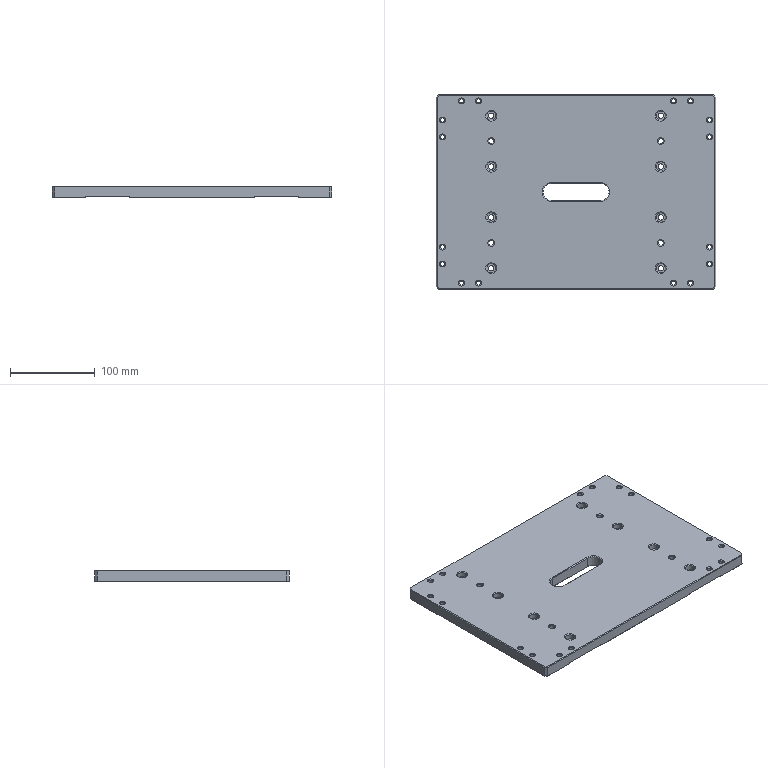Part | SolidWorks | features BaseBody 1 | 1 solid | 213 faces | box 330 x 230 x 14 mm | volume 980138 mm3 | cone 86 | cylinder 75 | plane 52 | commonest cylinder face diameters 5 x32 6.4 x16 11 x16 6 x8 20 x3